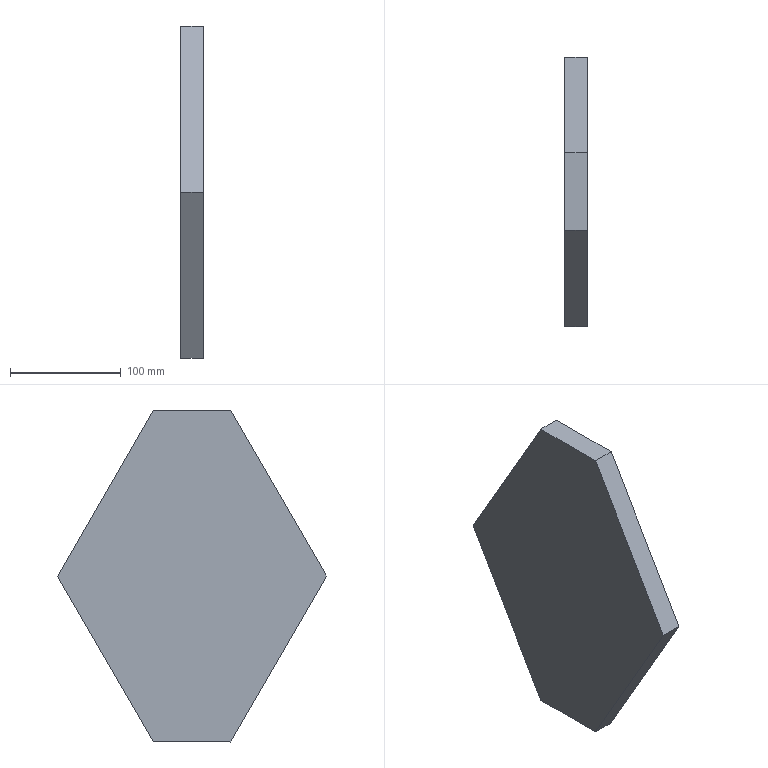Part | STEP file | Imported14 | 1 solid | 56 faces | box 20 x 243.205 x 300 mm | volume 845158 mm3 | plane 56